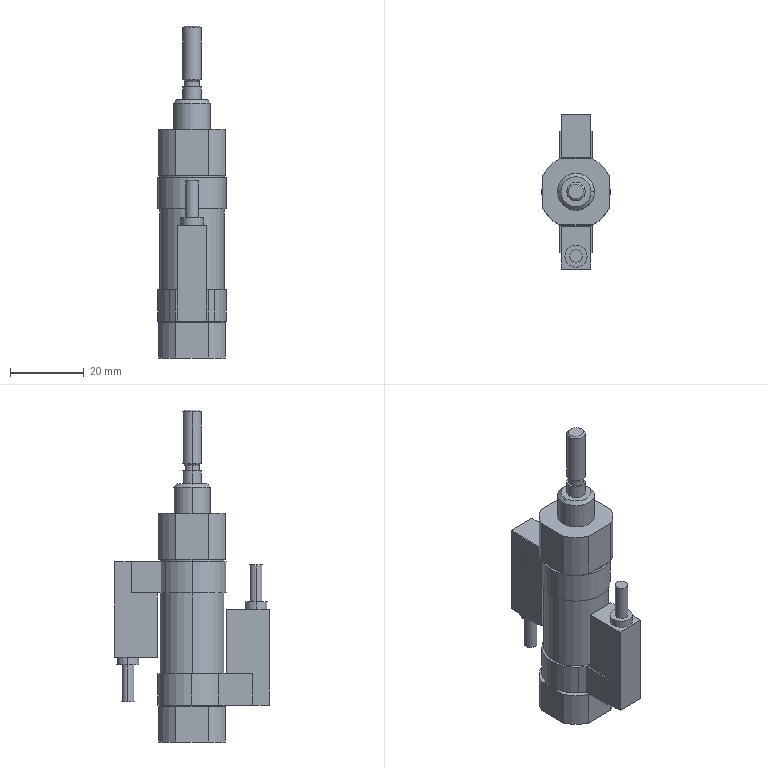Part | STEP file | Cylinder CDJ2B16-15-C73 (0) | 1 solid | 105 faces | box 18.6 x 41.8 x 90 mm | volume 22619 mm3 | plane 53 | cylinder 42 | cone 10 | commonest cylinder face diameters 18.6 x8 20 x8 17.4 x6 3.4 x4 4.13 x4 5 x4